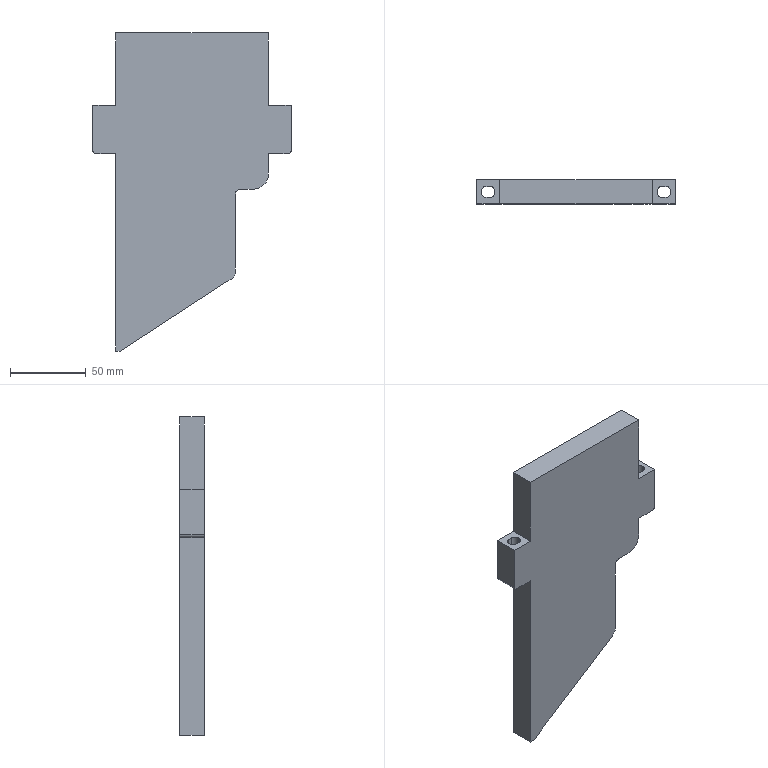Part | STEP file | 200 mesh_id2042 | 1 solid | 38 faces | box 131 x 16 x 210 mm | volume 283448 mm3 | plane 25 | cylinder 13 | commonest cylinder face diameters 6 x8 4 x2 6.5 x1 10 x1 20 x1
STEP:
#1=CARTESIAN_POINT('',(-16842.884,-3905.269,126.258));
#2=VERTEX_POINT('',#1);
#3=CARTESIAN_POINT('',(-16857.884,-3905.269,126.258));
#4=VERTEX_POINT('',#3);
#5=CARTESIAN_POINT('',(-16842.884,-3905.269,126.258));
#6=DIRECTION('',(-1.,0.,0.));
#7=VECTOR('',#6,1.);
#8=LINE('',#5,#7);
#9=EDGE_CURVE('',#2,#4,#8,.T.);
#10=ORIENTED_EDGE('',*,*,#9,.F.);
#11=CARTESIAN_POINT('',(-16842.884,-3889.269,126.258));
#12=VERTEX_POINT('',#11);
#13=CARTESIAN_POINT('',(-16842.884,-3889.269,126.258));
#14=DIRECTION('',(0.,-1.,0.));
#15=VECTOR('',#14,1.);
#16=LINE('',#13,#15);
#17=EDGE_CURVE('',#12,#2,#16,.T.);
#18=ORIENTED_EDGE('',*,*,#17,.F.);
#19=CARTESIAN_POINT('',(-16857.884,-3889.269,126.258));
#20=VERTEX_POINT('',#19);
#21=CARTESIAN_POINT('',(-16842.884,-3889.269,126.258));
#22=DIRECTION('',(-1.,0.,0.));
#23=VECTOR('',#22,1.);
#24=LINE('',#21,#23);
#25=EDGE_CURVE('',#12,#20,#24,.T.);
#26=ORIENTED_EDGE('',*,*,#25,.T.);
#27=CARTESIAN_POINT('',(-16857.884,-3889.269,126.258));
#28=DIRECTION('',(0.,-1.,0.));
#29=VECTOR('',#28,1.);
#30=LINE('',#27,#29);
#31=EDGE_CURVE('',#20,#4,#30,.T.);
#32=ORIENTED_EDGE('',*,*,#31,.T.);
#33=EDGE_LOOP('',(#10,#18,#26,#32));
#34=FACE_BOUND('',#33,.T.);
#35=CARTESIAN_POINT('',(-16851.884,-3893.769,126.258));
#36=VERTEX_POINT('',#35);
#37=CARTESIAN_POINT('',(-16848.884,-3893.769,126.258));
#38=VERTEX_POINT('',#37);
#39=CARTESIAN_POINT('',(-16842.884,-3893.769,126.258));
#40=DIRECTION('',(1.,0.,0.));
#41=VECTOR('',#40,1.);
#42=LINE('',#39,#41);
#43=EDGE_CURVE('',#36,#38,#42,.T.);
#44=ORIENTED_EDGE('',*,*,#43,.T.);
#45=CARTESIAN_POINT('',(-16845.884,-3896.769,126.258));
#46=VERTEX_POINT('',#45);
#47=CARTESIAN_POINT('',(-16848.884,-3896.769,126.258));
#48=DIRECTION('',(0.,0.,-1.));
#49=DIRECTION('',(-1.,0.,0.));
#50=AXIS2_PLACEMENT_3D('',#47,#48,#49);
#51=CIRCLE('',#50,3.);
#52=EDGE_CURVE('',#38,#46,#51,.T.);
#53=ORIENTED_EDGE('',*,*,#52,.T.);
#54=CARTESIAN_POINT('',(-16845.884,-3897.769,126.258));
#55=VERTEX_POINT('',#54);
#56=CARTESIAN_POINT('',(-16845.884,-3889.269,126.258));
#57=DIRECTION('',(0.,-1.,0.));
#58=VECTOR('',#57,1.);
#59=LINE('',#56,#58);
#60=EDGE_CURVE('',#46,#55,#59,.T.);
#61=ORIENTED_EDGE('',*,*,#60,.T.);
#62=CARTESIAN_POINT('',(-16848.884,-3900.769,126.258));
#63=VERTEX_POINT('',#62);
#64=CARTESIAN_POINT('',(-16848.884,-3897.769,126.258));
#65=DIRECTION('',(0.,0.,-1.));
#66=DIRECTION('',(-1.,0.,0.));
#67=AXIS2_PLACEMENT_3D('',#64,#65,#66);
#68=CIRCLE('',#67,3.);
#69=EDGE_CURVE('',#55,#63,#68,.T.);
#70=ORIENTED_EDGE('',*,*,#69,.T.);
#71=CARTESIAN_POINT('',(-16851.884,-3900.769,126.258));
#72=VERTEX_POINT('',#71);
#73=CARTESIAN_POINT('',(-16842.884,-3900.769,126.258));
#74=DIRECTION('',(-1.,0.,0.));
#75=VECTOR('',#74,1.);
#76=LINE('',#73,#75);
#77=EDGE_CURVE('',#63,#72,#76,.T.);
#78=ORIENTED_EDGE('',*,*,#77,.T.);
#79=CARTESIAN_POINT('',(-16854.884,-3897.769,126.258));
#80=VERTEX_POINT('',#79);
#81=CARTESIAN_POINT('',(-16851.884,-3897.769,126.258));
#82=DIRECTION('',(0.,0.,-1.));
#83=DIRECTION('',(-1.,0.,0.));
#84=AXIS2_PLACEMENT_3D('',#81,#82,#83);
#85=CIRCLE('',#84,3.);
#86=EDGE_CURVE('',#72,#80,#85,.T.);
#87=ORIENTED_EDGE('',*,*,#86,.T.);
#88=CARTESIAN_POINT('',(-16854.884,-3896.769,126.258));
#89=VERTEX_POINT('',#88);
#90=CARTESIAN_POINT('',(-16854.884,-3889.269,126.258));
#91=DIRECTION('',(0.,1.,0.));
#92=VECTOR('',#91,1.);
#93=LINE('',#90,#92);
#94=EDGE_CURVE('',#80,#89,#93,.T.);
#95=ORIENTED_EDGE('',*,*,#94,.T.);
#96=CARTESIAN_POINT('',(-16851.884,-3896.769,126.258));
#97=DIRECTION('',(0.,0.,-1.));
#98=DIRECTION('',(-1.,0.,0.));
#99=AXIS2_PLACEMENT_3D('',#96,#97,#98);
#100=CIRCLE('',#99,3.);
#101=EDGE_CURVE('',#89,#36,#100,.T.);
#102=ORIENTED_EDGE('',*,*,#101,.T.);
#103=EDGE_LOOP('',(#44,#53,#61,#70,#78,#87,#95,#102));
#104=FACE_BOUND('',#103,.T.);
#105=CARTESIAN_POINT('',(-16842.884,-3889.269,126.258));
#106=DIRECTION('',(0.,0.,-1.));
#107=DIRECTION('',(0.,-1.,0.));
#108=AXIS2_PLACEMENT_3D('',#105,#106,#107);
#109=PLANE('',#108);
#110=ADVANCED_FACE('',(#34,#104),#109,.F.);
#111=CARTESIAN_POINT('',(-16726.884,-3905.269,126.258));
#112=VERTEX_POINT('',#111);
#113=CARTESIAN_POINT('',(-16741.884,-3905.269,126.258));
#114=VERTEX_POINT('',#113);
#115=CARTESIAN_POINT('',(-16726.884,-3905.269,126.258));
#116=DIRECTION('',(-1.,0.,0.));
#117=VECTOR('',#116,1.);
#118=LINE('',#115,#117);
#119=EDGE_CURVE('',#112,#114,#118,.T.);
#120=ORIENTED_EDGE('',*,*,#119,.F.);
#121=CARTESIAN_POINT('',(-16726.884,-3889.269,126.258));
#122=VERTEX_POINT('',#121);
#123=CARTESIAN_POINT('',(-16726.884,-3889.269,126.258));
#124=DIRECTION('',(0.,-1.,0.));
#125=VECTOR('',#124,1.);
#126=LINE('',#123,#125);
#127=EDGE_CURVE('',#122,#112,#126,.T.);
#128=ORIENTED_EDGE('',*,*,#127,.F.);
#129=CARTESIAN_POINT('',(-16741.884,-3889.269,126.258));
#130=VERTEX_POINT('',#129);
#131=CARTESIAN_POINT('',(-16726.884,-3889.269,126.258));
#132=DIRECTION('',(-1.,0.,0.));
#133=VECTOR('',#132,1.);
#134=LINE('',#131,#133);
#135=EDGE_CURVE('',#122,#130,#134,.T.);
#136=ORIENTED_EDGE('',*,*,#135,.T.);
#137=CARTESIAN_POINT('',(-16741.884,-3889.269,126.258));
#138=DIRECTION('',(0.,-1.,0.));
#139=VECTOR('',#138,1.);
#140=LINE('',#137,#139);
#141=EDGE_CURVE('',#130,#114,#140,.T.);
#142=ORIENTED_EDGE('',*,*,#141,.T.);
#143=EDGE_LOOP('',(#120,#128,#136,#142));
#144=FACE_BOUND('',#143,.T.);
#145=CARTESIAN_POINT('',(-16738.884,-3897.769,126.258));
#146=VERTEX_POINT('',#145);
#147=CARTESIAN_POINT('',(-16738.884,-3896.769,126.258));
#148=VERTEX_POINT('',#147);
#149=CARTESIAN_POINT('',(-16738.884,-3889.269,126.258));
#150=DIRECTION('',(0.,1.,0.));
#151=VECTOR('',#150,1.);
#152=LINE('',#149,#151);
#153=EDGE_CURVE('',#146,#148,#152,.T.);
#154=ORIENTED_EDGE('',*,*,#153,.T.);
#155=CARTESIAN_POINT('',(-16735.884,-3893.769,126.258));
#156=VERTEX_POINT('',#155);
#157=CARTESIAN_POINT('',(-16735.884,-3896.769,126.258));
#158=DIRECTION('',(0.,0.,-1.));
#159=DIRECTION('',(-1.,0.,0.));
#160=AXIS2_PLACEMENT_3D('',#157,#158,#159);
#161=CIRCLE('',#160,3.);
#162=EDGE_CURVE('',#148,#156,#161,.T.);
#163=ORIENTED_EDGE('',*,*,#162,.T.);
#164=CARTESIAN_POINT('',(-16732.884,-3893.769,126.258));
#165=VERTEX_POINT('',#164);
#166=CARTESIAN_POINT('',(-16726.884,-3893.769,126.258));
#167=DIRECTION('',(1.,0.,0.));
#168=VECTOR('',#167,1.);
#169=LINE('',#166,#168);
#170=EDGE_CURVE('',#156,#165,#169,.T.);
#171=ORIENTED_EDGE('',*,*,#170,.T.);
#172=CARTESIAN_POINT('',(-16729.884,-3896.769,126.258));
#173=VERTEX_POINT('',#172);
#174=CARTESIAN_POINT('',(-16732.884,-3896.769,126.258));
#175=DIRECTION('',(0.,0.,-1.));
#176=DIRECTION('',(-1.,0.,0.));
#177=AXIS2_PLACEMENT_3D('',#174,#175,#176);
#178=CIRCLE('',#177,3.);
#179=EDGE_CURVE('',#165,#173,#178,.T.);
#180=ORIENTED_EDGE('',*,*,#179,.T.);
#181=CARTESIAN_POINT('',(-16729.884,-3897.769,126.258));
#182=VERTEX_POINT('',#181);
#183=CARTESIAN_POINT('',(-16729.884,-3889.269,126.258));
#184=DIRECTION('',(0.,-1.,0.));
#185=VECTOR('',#184,1.);
#186=LINE('',#183,#185);
#187=EDGE_CURVE('',#173,#182,#186,.T.);
#188=ORIENTED_EDGE('',*,*,#187,.T.);
#189=CARTESIAN_POINT('',(-16732.884,-3900.769,126.258));
#190=VERTEX_POINT('',#189);
#191=CARTESIAN_POINT('',(-16732.884,-3897.769,126.258));
#192=DIRECTION('',(0.,0.,-1.));
#193=DIRECTION('',(-1.,0.,0.));
#194=AXIS2_PLACEMENT_3D('',#191,#192,#193);
#195=CIRCLE('',#194,3.);
#196=EDGE_CURVE('',#182,#190,#195,.T.);
#197=ORIENTED_EDGE('',*,*,#196,.T.);
#198=CARTESIAN_POINT('',(-16735.884,-3900.769,126.258));
#199=VERTEX_POINT('',#198);
#200=CARTESIAN_POINT('',(-16726.884,-3900.769,126.258));
#201=DIRECTION('',(-1.,0.,0.));
#202=VECTOR('',#201,1.);
#203=LINE('',#200,#202);
#204=EDGE_CURVE('',#190,#199,#203,.T.);
#205=ORIENTED_EDGE('',*,*,#204,.T.);
#206=CARTESIAN_POINT('',(-16735.884,-3897.769,126.258));
#207=DIRECTION('',(0.,0.,-1.));
#208=DIRECTION('',(-1.,0.,0.));
#209=AXIS2_PLACEMENT_3D('',#206,#207,#208);
#210=CIRCLE('',#209,3.);
#211=EDGE_CURVE('',#199,#146,#210,.T.);
#212=ORIENTED_EDGE('',*,*,#211,.T.);
#213=EDGE_LOOP('',(#154,#163,#171,#180,#188,#197,#205,#212));
#214=FACE_BOUND('',#213,.T.);
#215=CARTESIAN_POINT('',(-16726.884,-3889.269,126.258));
#216=DIRECTION('',(0.,0.,-1.));
#217=DIRECTION('',(0.,-1.,0.));
#218=AXIS2_PLACEMENT_3D('',#215,#216,#217);
#219=PLANE('',#218);
#220=ADVANCED_FACE('',(#144,#214),#219,.F.);
#221=CARTESIAN_POINT('',(-16763.684,-3905.269,67.499));
#222=VERTEX_POINT('',#221);
#223=CARTESIAN_POINT('',(-16760.434,-3905.269,70.749));
#224=VERTEX_POINT('',#223);
#225=CARTESIAN_POINT('',(-16760.434,-3905.269,67.499));
#226=DIRECTION('',(0.,1.,0.));
#227=DIRECTION('',(0.,0.,-1.));
#228=AXIS2_PLACEMENT_3D('',#225,#226,#227);
#229=CIRCLE('',#228,3.25);
#230=EDGE_CURVE('',#222,#224,#229,.T.);
#231=ORIENTED_EDGE('',*,*,#230,.F.);
#232=CARTESIAN_POINT('',(-16763.684,-3889.269,67.499));
#233=VERTEX_POINT('',#232);
#234=CARTESIAN_POINT('',(-16763.684,-3889.269,67.499));
#235=DIRECTION('',(0.,-1.,0.));
#236=VECTOR('',#235,1.);
#237=LINE('',#234,#236);
#238=EDGE_CURVE('',#233,#222,#237,.T.);
#239=ORIENTED_EDGE('',*,*,#238,.F.);
#240=CARTESIAN_POINT('',(-16760.434,-3889.269,70.749));
#241=VERTEX_POINT('',#240);
#242=CARTESIAN_POINT('',(-16760.434,-3889.269,67.499));
#243=DIRECTION('',(0.,1.,0.));
#244=DIRECTION('',(0.,0.,-1.));
#245=AXIS2_PLACEMENT_3D('',#242,#243,#244);
#246=CIRCLE('',#245,3.25);
#247=EDGE_CURVE('',#233,#241,#246,.T.);
#248=ORIENTED_EDGE('',*,*,#247,.T.);
#249=CARTESIAN_POINT('',(-16760.434,-3889.269,70.749));
#250=DIRECTION('',(0.,-1.,0.));
#251=VECTOR('',#250,1.);
#252=LINE('',#249,#251);
#253=EDGE_CURVE('',#241,#224,#252,.T.);
#254=ORIENTED_EDGE('',*,*,#253,.T.);
#255=EDGE_LOOP('',(#231,#239,#248,#254));
#256=FACE_OUTER_BOUND('',#255,.T.);
#257=CARTESIAN_POINT('',(-16760.434,-3889.269,67.499));
#258=DIRECTION('',(0.,-1.,0.));
#259=DIRECTION('',(-1.,0.,0.));
#260=AXIS2_PLACEMENT_3D('',#257,#258,#259);
#261=CYLINDRICAL_SURFACE('',#260,3.25);
#262=ADVANCED_FACE('',(#256),#261,.F.);
#263=CARTESIAN_POINT('',(-16751.884,-3889.269,70.749));
#264=VERTEX_POINT('',#263);
#265=CARTESIAN_POINT('',(-16760.434,-3889.269,70.749));
#266=DIRECTION('',(1.,0.,0.));
#267=VECTOR('',#266,1.);
#268=LINE('',#265,#267);
#269=EDGE_CURVE('',#241,#264,#268,.T.);
#270=ORIENTED_EDGE('',*,*,#269,.T.);
#271=CARTESIAN_POINT('',(-16751.884,-3905.269,70.749));
#272=VERTEX_POINT('',#271);
#273=CARTESIAN_POINT('',(-16751.884,-3889.269,70.749));
#274=DIRECTION('',(0.,-1.,0.));
#275=VECTOR('',#274,1.);
#276=LINE('',#273,#275);
#277=EDGE_CURVE('',#264,#272,#276,.T.);
#278=ORIENTED_EDGE('',*,*,#277,.T.);
#279=CARTESIAN_POINT('',(-16760.434,-3905.269,70.749));
#280=DIRECTION('',(1.,0.,0.));
#281=VECTOR('',#280,1.);
#282=LINE('',#279,#281);
#283=EDGE_CURVE('',#224,#272,#282,.T.);
#284=ORIENTED_EDGE('',*,*,#283,.F.);
#285=ORIENTED_EDGE('',*,*,#253,.F.);
#286=EDGE_LOOP('',(#270,#278,#284,#285));
#287=FACE_OUTER_BOUND('',#286,.T.);
#288=CARTESIAN_POINT('',(-16760.434,-3889.269,70.749));
#289=DIRECTION('',(0.,0.,1.));
#290=DIRECTION('',(-1.,0.,0.));
#291=AXIS2_PLACEMENT_3D('',#288,#289,#290);
#292=PLANE('',#291);
#293=ADVANCED_FACE('',(#287),#292,.F.);
#294=CARTESIAN_POINT('',(-16741.884,-3905.269,80.749));
#295=VERTEX_POINT('',#294);
#296=CARTESIAN_POINT('',(-16741.884,-3905.269,94.258));
#297=VERTEX_POINT('',#296);
#298=CARTESIAN_POINT('',(-16741.884,-3905.269,72.499));
#299=DIRECTION('',(0.,0.,1.));
#300=VECTOR('',#299,1.);
#301=LINE('',#298,#300);
#302=EDGE_CURVE('',#295,#297,#301,.T.);
#303=ORIENTED_EDGE('',*,*,#302,.F.);
#304=CARTESIAN_POINT('',(-16741.884,-3889.269,80.749));
#305=VERTEX_POINT('',#304);
#306=CARTESIAN_POINT('',(-16741.884,-3889.269,80.749));
#307=DIRECTION('',(0.,1.,0.));
#308=VECTOR('',#307,1.);
#309=LINE('',#306,#308);
#310=EDGE_CURVE('',#295,#305,#309,.T.);
#311=ORIENTED_EDGE('',*,*,#310,.T.);
#312=CARTESIAN_POINT('',(-16741.884,-3889.269,94.258));
#313=VERTEX_POINT('',#312);
#314=CARTESIAN_POINT('',(-16741.884,-3889.269,72.499));
#315=DIRECTION('',(0.,0.,1.));
#316=VECTOR('',#315,1.);
#317=LINE('',#314,#316);
#318=EDGE_CURVE('',#305,#313,#317,.T.);
#319=ORIENTED_EDGE('',*,*,#318,.T.);
#320=CARTESIAN_POINT('',(-16741.884,-3889.269,94.258));
#321=DIRECTION('',(0.,-1.,0.));
#322=VECTOR('',#321,1.);
#323=LINE('',#320,#322);
#324=EDGE_CURVE('',#313,#297,#323,.T.);
#325=ORIENTED_EDGE('',*,*,#324,.T.);
#326=EDGE_LOOP('',(#303,#311,#319,#325));
#327=FACE_OUTER_BOUND('',#326,.T.);
#328=CARTESIAN_POINT('',(-16741.884,-3889.269,72.499));
#329=DIRECTION('',(-1.,0.,0.));
#330=DIRECTION('',(0.,1.,0.));
#331=AXIS2_PLACEMENT_3D('',#328,#329,#330);
#332=PLANE('',#331);
#333=ADVANCED_FACE('',(#327),#332,.F.);
#334=CARTESIAN_POINT('',(-16735.884,-3900.769,94.258));
#335=VERTEX_POINT('',#334);
#336=CARTESIAN_POINT('',(-16738.884,-3897.769,94.258));
#337=VERTEX_POINT('',#336);
#338=CARTESIAN_POINT('',(-16735.884,-3897.769,94.258));
#339=DIRECTION('',(0.,0.,-1.));
#340=DIRECTION('',(1.,0.,0.));
#341=AXIS2_PLACEMENT_3D('',#338,#339,#340);
#342=CIRCLE('',#341,3.);
#343=EDGE_CURVE('',#335,#337,#342,.T.);
#344=ORIENTED_EDGE('',*,*,#343,.F.);
#345=CARTESIAN_POINT('',(-16732.884,-3900.769,94.258));
#346=VERTEX_POINT('',#345);
#347=CARTESIAN_POINT('',(-16741.884,-3900.769,94.258));
#348=DIRECTION('',(-1.,0.,0.));
#349=VECTOR('',#348,1.);
#350=LINE('',#347,#349);
#351=EDGE_CURVE('',#346,#335,#350,.T.);
#352=ORIENTED_EDGE('',*,*,#351,.F.);
#353=CARTESIAN_POINT('',(-16729.884,-3897.769,94.258));
#354=VERTEX_POINT('',#353);
#355=CARTESIAN_POINT('',(-16732.884,-3897.769,94.258));
#356=DIRECTION('',(0.,0.,-1.));
#357=DIRECTION('',(1.,0.,0.));
#358=AXIS2_PLACEMENT_3D('',#355,#356,#357);
#359=CIRCLE('',#358,3.);
#360=EDGE_CURVE('',#354,#346,#359,.T.);
#361=ORIENTED_EDGE('',*,*,#360,.F.);
#362=CARTESIAN_POINT('',(-16729.884,-3896.769,94.258));
#363=VERTEX_POINT('',#362);
#364=CARTESIAN_POINT('',(-16729.884,-3889.269,94.258));
#365=DIRECTION('',(0.,-1.,0.));
#366=VECTOR('',#365,1.);
#367=LINE('',#364,#366);
#368=EDGE_CURVE('',#363,#354,#367,.T.);
#369=ORIENTED_EDGE('',*,*,#368,.F.);
#370=CARTESIAN_POINT('',(-16732.884,-3893.769,94.258));
#371=VERTEX_POINT('',#370);
#372=CARTESIAN_POINT('',(-16732.884,-3896.769,94.258));
#373=DIRECTION('',(0.,0.,-1.));
#374=DIRECTION('',(1.,0.,0.));
#375=AXIS2_PLACEMENT_3D('',#372,#373,#374);
#376=CIRCLE('',#375,3.);
#377=EDGE_CURVE('',#371,#363,#376,.T.);
#378=ORIENTED_EDGE('',*,*,#377,.F.);
#379=CARTESIAN_POINT('',(-16735.884,-3893.769,94.258));
#380=VERTEX_POINT('',#379);
#381=CARTESIAN_POINT('',(-16741.884,-3893.769,94.258));
#382=DIRECTION('',(1.,0.,0.));
#383=VECTOR('',#382,1.);
#384=LINE('',#381,#383);
#385=EDGE_CURVE('',#380,#371,#384,.T.);
#386=ORIENTED_EDGE('',*,*,#385,.F.);
#387=CARTESIAN_POINT('',(-16738.884,-3896.769,94.258));
#388=VERTEX_POINT('',#387);
#389=CARTESIAN_POINT('',(-16735.884,-3896.769,94.258));
#390=DIRECTION('',(0.,0.,-1.));
#391=DIRECTION('',(1.,0.,0.));
#392=AXIS2_PLACEMENT_3D('',#389,#390,#391);
#393=CIRCLE('',#392,3.);
#394=EDGE_CURVE('',#388,#380,#393,.T.);
#395=ORIENTED_EDGE('',*,*,#394,.F.);
#396=CARTESIAN_POINT('',(-16738.884,-3889.269,94.258));
#397=DIRECTION('',(0.,1.,0.));
#398=VECTOR('',#397,1.);
#399=LINE('',#396,#398);
#400=EDGE_CURVE('',#337,#388,#399,.T.);
#401=ORIENTED_EDGE('',*,*,#400,.F.);
#402=EDGE_LOOP('',(#344,#352,#361,#369,#378,#386,#395,#401));
#403=FACE_BOUND('',#402,.T.);
#404=CARTESIAN_POINT('',(-16728.884,-3889.269,94.258));
#405=VERTEX_POINT('',#404);
#406=CARTESIAN_POINT('',(-16741.884,-3889.269,94.258));
#407=DIRECTION('',(1.,0.,0.));
#408=VECTOR('',#407,1.);
#409=LINE('',#406,#408);
#410=EDGE_CURVE('',#313,#405,#409,.T.);
#411=ORIENTED_EDGE('',*,*,#410,.T.);
#412=CARTESIAN_POINT('',(-16728.884,-3905.269,94.258));
#413=VERTEX_POINT('',#412);
#414=CARTESIAN_POINT('',(-16728.884,-3889.269,94.258));
#415=DIRECTION('',(0.,-1.,0.));
#416=VECTOR('',#415,1.);
#417=LINE('',#414,#416);
#418=EDGE_CURVE('',#405,#413,#417,.T.);
#419=ORIENTED_EDGE('',*,*,#418,.T.);
#420=CARTESIAN_POINT('',(-16741.884,-3905.269,94.258));
#421=DIRECTION('',(1.,0.,0.));
#422=VECTOR('',#421,1.);
#423=LINE('',#420,#422);
#424=EDGE_CURVE('',#297,#413,#423,.T.);
#425=ORIENTED_EDGE('',*,*,#424,.F.);
#426=ORIENTED_EDGE('',*,*,#324,.F.);
#427=EDGE_LOOP('',(#411,#419,#425,#426));
#428=FACE_BOUND('',#427,.T.);
#429=CARTESIAN_POINT('',(-16741.884,-3889.269,94.258));
#430=DIRECTION('',(0.,0.,1.));
#431=DIRECTION('',(0.,1.,0.));
#432=AXIS2_PLACEMENT_3D('',#429,#430,#431);
#433=PLANE('',#432);
#434=ADVANCED_FACE('',(#403,#428),#433,.F.);
#435=CARTESIAN_POINT('',(-16726.884,-3905.269,96.258));
#436=VERTEX_POINT('',#435);
#437=CARTESIAN_POINT('',(-16726.884,-3905.269,94.258));
#438=DIRECTION('',(0.,0.,1.));
#439=VECTOR('',#438,1.);
#440=LINE('',#437,#439);
#441=EDGE_CURVE('',#436,#112,#440,.T.);
#442=ORIENTED_EDGE('',*,*,#441,.F.);
#443=CARTESIAN_POINT('',(-16726.884,-3889.269,96.258));
#444=VERTEX_POINT('',#443);
#445=CARTESIAN_POINT('',(-16726.884,-3889.269,96.258));
#446=DIRECTION('',(0.,1.,0.));
#447=VECTOR('',#446,1.);
#448=LINE('',#445,#447);
#449=EDGE_CURVE('',#436,#444,#448,.T.);
#450=ORIENTED_EDGE('',*,*,#449,.T.);
#451=CARTESIAN_POINT('',(-16726.884,-3889.269,94.258));
#452=DIRECTION('',(0.,0.,1.));
#453=VECTOR('',#452,1.);
#454=LINE('',#451,#453);
#455=EDGE_CURVE('',#444,#122,#454,.T.);
#456=ORIENTED_EDGE('',*,*,#455,.T.);
#457=ORIENTED_EDGE('',*,*,#127,.T.);
#458=EDGE_LOOP('',(#442,#450,#456,#457));
#459=FACE_OUTER_BOUND('',#458,.T.);
#460=CARTESIAN_POINT('',(-16726.884,-3889.269,94.258));
#461=DIRECTION('',(-1.,0.,0.));
#462=DIRECTION('',(0.,1.,0.));
#463=AXIS2_PLACEMENT_3D('',#460,#461,#462);
#464=PLANE('',#463);
#465=ADVANCED_FACE('',(#459),#464,.F.);
#466=CARTESIAN_POINT('',(-16741.884,-3905.269,173.87));
#467=VERTEX_POINT('',#466);
#468=CARTESIAN_POINT('',(-16741.884,-3905.269,124.258));
#469=DIRECTION('',(0.,0.,1.));
#470=VECTOR('',#469,1.);
#471=LINE('',#468,#470);
#472=EDGE_CURVE('',#114,#467,#471,.T.);
#473=ORIENTED_EDGE('',*,*,#472,.F.);
#474=ORIENTED_EDGE('',*,*,#141,.F.);
#475=CARTESIAN_POINT('',(-16741.884,-3889.269,173.87));
#476=VERTEX_POINT('',#475);
#477=CARTESIAN_POINT('',(-16741.884,-3889.269,124.258));
#478=DIRECTION('',(0.,0.,1.));
#479=VECTOR('',#478,1.);
#480=LINE('',#477,#479);
#481=EDGE_CURVE('',#130,#476,#480,.T.);
#482=ORIENTED_EDGE('',*,*,#481,.T.);
#483=CARTESIAN_POINT('',(-16741.884,-3889.269,173.87));
#484=DIRECTION('',(0.,-1.,0.));
#485=VECTOR('',#484,1.);
#486=LINE('',#483,#485);
#487=EDGE_CURVE('',#476,#467,#486,.T.);
#488=ORIENTED_EDGE('',*,*,#487,.T.);
#489=EDGE_LOOP('',(#473,#474,#482,#488));
#490=FACE_OUTER_BOUND('',#489,.T.);
#491=CARTESIAN_POINT('',(-16741.884,-3889.269,124.258));
#492=DIRECTION('',(-1.,0.,0.));
#493=DIRECTION('',(0.,1.,0.));
#494=AXIS2_PLACEMENT_3D('',#491,#492,#493);
#495=PLANE('',#494);
#496=ADVANCED_FACE('',(#490),#495,.F.);
#497=CARTESIAN_POINT('',(-16842.884,-3905.269,173.87));
#498=VERTEX_POINT('',#497);
#499=CARTESIAN_POINT('',(-16731.884,-3905.269,173.87));
#500=DIRECTION('',(-1.,0.,0.));
#501=VECTOR('',#500,1.);
#502=LINE('',#499,#501);
#503=EDGE_CURVE('',#467,#498,#502,.T.);
#504=ORIENTED_EDGE('',*,*,#503,.F.);
#505=ORIENTED_EDGE('',*,*,#487,.F.);
#506=CARTESIAN_POINT('',(-16842.884,-3889.269,173.87));
#507=VERTEX_POINT('',#506);
#508=CARTESIAN_POINT('',(-16731.884,-3889.269,173.87));
#509=DIRECTION('',(-1.,0.,0.));
#510=VECTOR('',#509,1.);
#511=LINE('',#508,#510);
#512=EDGE_CURVE('',#476,#507,#511,.T.);
#513=ORIENTED_EDGE('',*,*,#512,.T.);
#514=CARTESIAN_POINT('',(-16842.884,-3889.269,173.87));
#515=DIRECTION('',(0.,-1.,0.));
#516=VECTOR('',#515,1.);
#517=LINE('',#514,#516);
#518=EDGE_CURVE('',#507,#498,#517,.T.);
#519=ORIENTED_EDGE('',*,*,#518,.T.);
#520=EDGE_LOOP('',(#504,#505,#513,#519));
#521=FACE_OUTER_BOUND('',#520,.T.);
#522=CARTESIAN_POINT('',(-16731.884,-3889.269,173.87));
#523=DIRECTION('',(0.,0.,-1.));
#524=DIRECTION('',(0.,-1.,0.));
#525=AXIS2_PLACEMENT_3D('',#522,#523,#524);
#526=PLANE('',#525);
#527=ADVANCED_FACE('',(#521),#526,.F.);
#528=CARTESIAN_POINT('',(-16842.884,-3905.269,153.87));
#529=DIRECTION('',(0.,0.,-1.));
#530=VECTOR('',#529,1.);
#531=LINE('',#528,#530);
#532=EDGE_CURVE('',#498,#2,#531,.T.);
#533=ORIENTED_EDGE('',*,*,#532,.F.);
#534=ORIENTED_EDGE('',*,*,#518,.F.);
#535=CARTESIAN_POINT('',(-16842.884,-3889.269,153.87));
#536=DIRECTION('',(0.,0.,-1.));
#537=VECTOR('',#536,1.);
#538=LINE('',#535,#537);
#539=EDGE_CURVE('',#507,#12,#538,.T.);
#540=ORIENTED_EDGE('',*,*,#539,.T.);
#541=ORIENTED_EDGE('',*,*,#17,.T.);
#542=EDGE_LOOP('',(#533,#534,#540,#541));
#543=FACE_OUTER_BOUND('',#542,.T.);
#544=CARTESIAN_POINT('',(-16842.884,-3889.269,153.87));
#545=DIRECTION('',(1.,0.,0.));
#546=DIRECTION('',(0.,-1.,0.));
#547=AXIS2_PLACEMENT_3D('',#544,#545,#546);
#548=PLANE('',#547);
#549=ADVANCED_FACE('',(#543),#548,.F.);
#550=CARTESIAN_POINT('',(-16857.884,-3889.269,96.258));
#551=VERTEX_POINT('',#550);
#552=CARTESIAN_POINT('',(-16857.884,-3889.269,124.258));
#553=DIRECTION('',(0.,0.,-1.));
#554=VECTOR('',#553,1.);
#555=LINE('',#552,#554);
#556=EDGE_CURVE('',#20,#551,#555,.T.);
#557=ORIENTED_EDGE('',*,*,#556,.T.);
#558=CARTESIAN_POINT('',(-16857.884,-3905.269,96.258));
#559=VERTEX_POINT('',#558);
#560=CARTESIAN_POINT('',(-16857.884,-3889.269,96.258));
#561=DIRECTION('',(0.,-1.,0.));
#562=VECTOR('',#561,1.);
#563=LINE('',#560,#562);
#564=EDGE_CURVE('',#551,#559,#563,.T.);
#565=ORIENTED_EDGE('',*,*,#564,.T.);
#566=CARTESIAN_POINT('',(-16857.884,-3905.269,124.258));
#567=DIRECTION('',(0.,0.,-1.));
#568=VECTOR('',#567,1.);
#569=LINE('',#566,#568);
#570=EDGE_CURVE('',#4,#559,#569,.T.);
#571=ORIENTED_EDGE('',*,*,#570,.F.);
#572=ORIENTED_EDGE('',*,*,#31,.F.);
#573=EDGE_LOOP('',(#557,#565,#571,#572));
#574=FACE_OUTER_BOUND('',#573,.T.);
#575=CARTESIAN_POINT('',(-16857.884,-3889.269,124.258));
#576=DIRECTION('',(1.,0.,0.));
#577=DIRECTION('',(0.,-1.,0.));
#578=AXIS2_PLACEMENT_3D('',#575,#576,#577);
#579=PLANE('',#578);
#580=ADVANCED_FACE('',(#574),#579,.F.);
#581=CARTESIAN_POINT('',(-16854.884,-3896.769,94.258));
#582=VERTEX_POINT('',#581);
#583=CARTESIAN_POINT('',(-16851.884,-3893.769,94.258));
#584=VERTEX_POINT('',#583);
#585=CARTESIAN_POINT('',(-16851.884,-3896.769,94.258));
#586=DIRECTION('',(0.,0.,-1.));
#587=DIRECTION('',(1.,0.,0.));
#588=AXIS2_PLACEMENT_3D('',#585,#586,#587);
#589=CIRCLE('',#588,3.);
#590=EDGE_CURVE('',#582,#584,#589,.T.);
#591=ORIENTED_EDGE('',*,*,#590,.F.);
#592=CARTESIAN_POINT('',(-16854.884,-3897.769,94.258));
#593=VERTEX_POINT('',#592);
#594=CARTESIAN_POINT('',(-16854.884,-3889.269,94.258));
#595=DIRECTION('',(0.,1.,0.));
#596=VECTOR('',#595,1.);
#597=LINE('',#594,#596);
#598=EDGE_CURVE('',#593,#582,#597,.T.);
#599=ORIENTED_EDGE('',*,*,#598,.F.);
#600=CARTESIAN_POINT('',(-16851.884,-3900.769,94.258));
#601=VERTEX_POINT('',#600);
#602=CARTESIAN_POINT('',(-16851.884,-3897.769,94.258));
#603=DIRECTION('',(0.,0.,-1.));
#604=DIRECTION('',(1.,0.,0.));
#605=AXIS2_PLACEMENT_3D('',#602,#603,#604);
#606=CIRCLE('',#605,3.);
#607=EDGE_CURVE('',#601,#593,#606,.T.);
#608=ORIENTED_EDGE('',*,*,#607,.F.);
#609=CARTESIAN_POINT('',(-16848.884,-3900.769,94.258));
#610=VERTEX_POINT('',#609);
#611=CARTESIAN_POINT('',(-16857.884,-3900.769,94.258));
#612=DIRECTION('',(-1.,0.,0.));
#613=VECTOR('',#612,1.);
#614=LINE('',#611,#613);
#615=EDGE_CURVE('',#610,#601,#614,.T.);
#616=ORIENTED_EDGE('',*,*,#615,.F.);
#617=CARTESIAN_POINT('',(-16845.884,-3897.769,94.258));
#618=VERTEX_POINT('',#617);
#619=CARTESIAN_POINT('',(-16848.884,-3897.769,94.258));
#620=DIRECTION('',(0.,0.,-1.));
#621=DIRECTION('',(1.,0.,0.));
#622=AXIS2_PLACEMENT_3D('',#619,#620,#621);
#623=CIRCLE('',#622,3.);
#624=EDGE_CURVE('',#618,#610,#623,.T.);
#625=ORIENTED_EDGE('',*,*,#624,.F.);
#626=CARTESIAN_POINT('',(-16845.884,-3896.769,94.258));
#627=VERTEX_POINT('',#626);
#628=CARTESIAN_POINT('',(-16845.884,-3889.269,94.258));
#629=DIRECTION('',(0.,-1.,0.));
#630=VECTOR('',#629,1.);
#631=LINE('',#628,#630);
#632=EDGE_CURVE('',#627,#618,#631,.T.);
#633=ORIENTED_EDGE('',*,*,#632,.F.);
#634=CARTESIAN_POINT('',(-16848.884,-3893.769,94.258));
#635=VERTEX_POINT('',#634);
#636=CARTESIAN_POINT('',(-16848.884,-3896.769,94.258));
#637=DIRECTION('',(0.,0.,-1.));
#638=DIRECTION('',(1.,0.,0.));
#639=AXIS2_PLACEMENT_3D('',#636,#637,#638);
#640=CIRCLE('',#639,3.);
#641=EDGE_CURVE('',#635,#627,#640,.T.);
#642=ORIENTED_EDGE('',*,*,#641,.F.);
#643=CARTESIAN_POINT('',(-16857.884,-3893.769,94.258));
#644=DIRECTION('',(1.,0.,0.));
#645=VECTOR('',#644,1.);
#646=LINE('',#643,#645);
#647=EDGE_CURVE('',#584,#635,#646,.T.);
#648=ORIENTED_EDGE('',*,*,#647,.F.);
#649=EDGE_LOOP('',(#591,#599,#608,#616,#625,#633,#642,#648));
#650=FACE_BOUND('',#649,.T.);
#651=CARTESIAN_POINT('',(-16855.884,-3905.269,94.258));
#652=VERTEX_POINT('',#651);
#653=CARTESIAN_POINT('',(-16842.884,-3905.269,94.258));
#654=VERTEX_POINT('',#653);
#655=CARTESIAN_POINT('',(-16857.884,-3905.269,94.258));
#656=DIRECTION('',(1.,0.,0.));
#657=VECTOR('',#656,1.);
#658=LINE('',#655,#657);
#659=EDGE_CURVE('',#652,#654,#658,.T.);
#660=ORIENTED_EDGE('',*,*,#659,.F.);
#661=CARTESIAN_POINT('',(-16855.884,-3889.269,94.258));
#662=VERTEX_POINT('',#661);
#663=CARTESIAN_POINT('',(-16855.884,-3889.269,94.258));
#664=DIRECTION('',(0.,1.,0.));
#665=VECTOR('',#664,1.);
#666=LINE('',#663,#665);
#667=EDGE_CURVE('',#652,#662,#666,.T.);
#668=ORIENTED_EDGE('',*,*,#667,.T.);
#669=CARTESIAN_POINT('',(-16842.884,-3889.269,94.258));
#670=VERTEX_POINT('',#669);
#671=CARTESIAN_POINT('',(-16857.884,-3889.269,94.258));
#672=DIRECTION('',(1.,0.,0.));
#673=VECTOR('',#672,1.);
#674=LINE('',#671,#673);
#675=EDGE_CURVE('',#662,#670,#674,.T.);
#676=ORIENTED_EDGE('',*,*,#675,.T.);
#677=CARTESIAN_POINT('',(-16842.884,-3889.269,94.258));
#678=DIRECTION('',(0.,-1.,0.));
#679=VECTOR('',#678,1.);
#680=LINE('',#677,#679);
#681=EDGE_CURVE('',#670,#654,#680,.T.);
#682=ORIENTED_EDGE('',*,*,#681,.T.);
#683=EDGE_LOOP('',(#660,#668,#676,#682));
#684=FACE_BOUND('',#683,.T.);
#685=CARTESIAN_POINT('',(-16857.884,-3889.269,94.258));
#686=DIRECTION('',(0.,0.,1.));
#687=DIRECTION('',(0.,1.,0.));
#688=AXIS2_PLACEMENT_3D('',#685,#686,#687);
#689=PLANE('',#688);
#690=ADVANCED_FACE('',(#650,#684),#689,.F.);
#691=CARTESIAN_POINT('',(-16842.884,-3905.269,-36.13));
#692=VERTEX_POINT('',#691);
#693=CARTESIAN_POINT('',(-16842.884,-3905.269,94.258));
#694=DIRECTION('',(0.,0.,-1.));
#695=VECTOR('',#694,1.);
#696=LINE('',#693,#695);
#697=EDGE_CURVE('',#654,#692,#696,.T.);
#698=ORIENTED_EDGE('',*,*,#697,.F.);
#699=ORIENTED_EDGE('',*,*,#681,.F.);
#700=CARTESIAN_POINT('',(-16842.884,-3889.269,-36.13));
#701=VERTEX_POINT('',#700);
#702=CARTESIAN_POINT('',(-16842.884,-3889.269,94.258));
#703=DIRECTION('',(0.,0.,-1.));
#704=VECTOR('',#703,1.);
#705=LINE('',#702,#704);
#706=EDGE_CURVE('',#670,#701,#705,.T.);
#707=ORIENTED_EDGE('',*,*,#706,.T.);
#708=CARTESIAN_POINT('',(-16842.884,-3889.269,-36.13));
#709=DIRECTION('',(0.,-1.,0.));
#710=VECTOR('',#709,1.);
#711=LINE('',#708,#710);
#712=EDGE_CURVE('',#701,#692,#711,.T.);
#713=ORIENTED_EDGE('',*,*,#712,.T.);
#714=EDGE_LOOP('',(#698,#699,#707,#713));
#715=FACE_OUTER_BOUND('',#714,.T.);
#716=CARTESIAN_POINT('',(-16842.884,-3889.269,94.258));
#717=DIRECTION('',(1.,0.,0.));
#718=DIRECTION('',(0.,-1.,0.));
#719=AXIS2_PLACEMENT_3D('',#716,#717,#718);
#720=PLANE('',#719);
#721=ADVANCED_FACE('',(#715),#720,.F.);
#722=CARTESIAN_POINT('',(-16839.804,-3905.269,-36.13));
#723=VERTEX_POINT('',#722);
#724=CARTESIAN_POINT('',(-16842.884,-3905.269,-36.13));
#725=DIRECTION('',(1.,0.,0.));
#726=VECTOR('',#725,1.);
#727=LINE('',#724,#726);
#728=EDGE_CURVE('',#692,#723,#727,.T.);
#729=ORIENTED_EDGE('',*,*,#728,.F.);
#730=ORIENTED_EDGE('',*,*,#712,.F.);
#731=CARTESIAN_POINT('',(-16839.804,-3889.269,-36.13));
#732=VERTEX_POINT('',#731);
#733=CARTESIAN_POINT('',(-16842.884,-3889.269,-36.13));
#734=DIRECTION('',(1.,0.,0.));
#735=VECTOR('',#734,1.);
#736=LINE('',#733,#735);
#737=EDGE_CURVE('',#701,#732,#736,.T.);
#738=ORIENTED_EDGE('',*,*,#737,.T.);
#739=CARTESIAN_POINT('',(-16839.804,-3889.269,-36.13));
#740=DIRECTION('',(0.,-1.,0.));
#741=VECTOR('',#740,1.);
#742=LINE('',#739,#741);
#743=EDGE_CURVE('',#732,#723,#742,.T.);
#744=ORIENTED_EDGE('',*,*,#743,.T.);
#745=EDGE_LOOP('',(#729,#730,#738,#744));
#746=FACE_OUTER_BOUND('',#745,.T.);
#747=CARTESIAN_POINT('',(-16842.884,-3889.269,-36.13));
#748=DIRECTION('',(0.,0.,1.));
#749=DIRECTION('',(0.,1.,0.));
#750=AXIS2_PLACEMENT_3D('',#747,#748,#749);
#751=PLANE('',#750);
#752=ADVANCED_FACE('',(#746),#751,.F.);
#753=CARTESIAN_POINT('',(-16765.961,-3889.269,11.825));
#754=VERTEX_POINT('',#753);
#755=CARTESIAN_POINT('',(-16839.804,-3889.269,-36.13));
#756=DIRECTION('',(0.8387,0.,0.5446));
#757=VECTOR('',#756,1.);
#758=LINE('',#755,#757);
#759=EDGE_CURVE('',#732,#754,#758,.T.);
#760=ORIENTED_EDGE('',*,*,#759,.T.);
#761=CARTESIAN_POINT('',(-16765.961,-3905.269,11.825));
#762=VERTEX_POINT('',#761);
#763=CARTESIAN_POINT('',(-16765.961,-3889.269,11.825));
#764=DIRECTION('',(0.,-1.,0.));
#765=VECTOR('',#764,1.);
#766=LINE('',#763,#765);
#767=EDGE_CURVE('',#754,#762,#766,.T.);
#768=ORIENTED_EDGE('',*,*,#767,.T.);
#769=CARTESIAN_POINT('',(-16839.804,-3905.269,-36.13));
#770=DIRECTION('',(0.8387,0.,0.5446));
#771=VECTOR('',#770,1.);
#772=LINE('',#769,#771);
#773=EDGE_CURVE('',#723,#762,#772,.T.);
#774=ORIENTED_EDGE('',*,*,#773,.F.);
#775=ORIENTED_EDGE('',*,*,#743,.F.);
#776=EDGE_LOOP('',(#760,#768,#774,#775));
#777=FACE_OUTER_BOUND('',#776,.T.);
#778=CARTESIAN_POINT('',(-16839.804,-3889.269,-36.13));
#779=DIRECTION('',(-0.5446,0.,0.8387));
#780=DIRECTION('',(-0.8387,0.,-0.5446));
#781=AXIS2_PLACEMENT_3D('',#778,#779,#780);
#782=PLANE('',#781);
#783=ADVANCED_FACE('',(#777),#782,.F.);
#784=CARTESIAN_POINT('',(-16763.684,-3905.269,16.018));
#785=VERTEX_POINT('',#784);
#786=CARTESIAN_POINT('',(-16763.684,-3905.269,53.944));
#787=DIRECTION('',(0.,0.,1.));
#788=VECTOR('',#787,1.);
#789=LINE('',#786,#788);
#790=EDGE_CURVE('',#785,#222,#789,.T.);
#791=ORIENTED_EDGE('',*,*,#790,.F.);
#792=CARTESIAN_POINT('',(-16763.684,-3889.269,16.018));
#793=VERTEX_POINT('',#792);
#794=CARTESIAN_POINT('',(-16763.684,-3889.269,16.018));
#795=DIRECTION('',(0.,1.,0.));
#796=VECTOR('',#795,1.);
#797=LINE('',#794,#796);
#798=EDGE_CURVE('',#785,#793,#797,.T.);
#799=ORIENTED_EDGE('',*,*,#798,.T.);
#800=CARTESIAN_POINT('',(-16763.684,-3889.269,53.944));
#801=DIRECTION('',(0.,0.,1.));
#802=VECTOR('',#801,1.);
#803=LINE('',#800,#802);
#804=EDGE_CURVE('',#793,#233,#803,.T.);
#805=ORIENTED_EDGE('',*,*,#804,.T.);
#806=ORIENTED_EDGE('',*,*,#238,.T.);
#807=EDGE_LOOP('',(#791,#799,#805,#806));
#808=FACE_OUTER_BOUND('',#807,.T.);
#809=CARTESIAN_POINT('',(-16763.684,-3889.269,53.944));
#810=DIRECTION('',(-1.,0.,0.));
#811=DIRECTION('',(0.,1.,0.));
#812=AXIS2_PLACEMENT_3D('',#809,#810,#811);
#813=PLANE('',#812);
#814=ADVANCED_FACE('',(#808),#813,.F.);
#815=ORIENTED_EDGE('',*,*,#804,.F.);
#816=CARTESIAN_POINT('',(-16768.684,-3889.269,16.018));
#817=DIRECTION('',(0.,1.,0.));
#818=DIRECTION('',(0.,0.,-1.));
#819=AXIS2_PLACEMENT_3D('',#816,#817,#818);
#820=CIRCLE('',#819,5.);
#821=EDGE_CURVE('',#793,#754,#820,.T.);
#822=ORIENTED_EDGE('',*,*,#821,.T.);
#823=ORIENTED_EDGE('',*,*,#759,.F.);
#824=ORIENTED_EDGE('',*,*,#737,.F.);
#825=ORIENTED_EDGE('',*,*,#706,.F.);
#826=ORIENTED_EDGE('',*,*,#675,.F.);
#827=CARTESIAN_POINT('',(-16855.884,-3889.269,96.258));
#828=DIRECTION('',(0.,1.,0.));
#829=DIRECTION('',(0.,0.,-1.));
#830=AXIS2_PLACEMENT_3D('',#827,#828,#829);
#831=CIRCLE('',#830,2.);
#832=EDGE_CURVE('',#662,#551,#831,.T.);
#833=ORIENTED_EDGE('',*,*,#832,.T.);
#834=ORIENTED_EDGE('',*,*,#556,.F.);
#835=ORIENTED_EDGE('',*,*,#25,.F.);
#836=ORIENTED_EDGE('',*,*,#539,.F.);
#837=ORIENTED_EDGE('',*,*,#512,.F.);
#838=ORIENTED_EDGE('',*,*,#481,.F.);
#839=ORIENTED_EDGE('',*,*,#135,.F.);
#840=ORIENTED_EDGE('',*,*,#455,.F.);
#841=CARTESIAN_POINT('',(-16728.884,-3889.269,96.258));
#842=DIRECTION('',(0.,1.,0.));
#843=DIRECTION('',(0.,0.,-1.));
#844=AXIS2_PLACEMENT_3D('',#841,#842,#843);
#845=CIRCLE('',#844,2.);
#846=EDGE_CURVE('',#444,#405,#845,.T.);
#847=ORIENTED_EDGE('',*,*,#846,.T.);
#848=ORIENTED_EDGE('',*,*,#410,.F.);
#849=ORIENTED_EDGE('',*,*,#318,.F.);
#850=CARTESIAN_POINT('',(-16751.884,-3889.269,80.749));
#851=DIRECTION('',(0.,1.,0.));
#852=DIRECTION('',(0.,0.,-1.));
#853=AXIS2_PLACEMENT_3D('',#850,#851,#852);
#854=CIRCLE('',#853,10.);
#855=EDGE_CURVE('',#305,#264,#854,.T.);
#856=ORIENTED_EDGE('',*,*,#855,.T.);
#857=ORIENTED_EDGE('',*,*,#269,.F.);
#858=ORIENTED_EDGE('',*,*,#247,.F.);
#859=EDGE_LOOP('',(#815,#822,#823,#824,#825,#826,#833,#834,#835,#836,#837,#838,#839,#840,#847,#848,#849,#856,#857,#858));
#860=FACE_OUTER_BOUND('',#859,.T.);
#861=CARTESIAN_POINT('',(-16760.434,-3889.269,67.499));
#862=DIRECTION('',(0.,-1.,0.));
#863=DIRECTION('',(-1.,0.,0.));
#864=AXIS2_PLACEMENT_3D('',#861,#862,#863);
#865=PLANE('',#864);
#866=ADVANCED_FACE('',(#860),#865,.F.);
#867=ORIENTED_EDGE('',*,*,#773,.T.);
#868=CARTESIAN_POINT('',(-16768.684,-3905.269,16.018));
#869=DIRECTION('',(0.,-1.,0.));
#870=DIRECTION('',(0.,0.,-1.));
#871=AXIS2_PLACEMENT_3D('',#868,#869,#870);
#872=CIRCLE('',#871,5.);
#873=EDGE_CURVE('',#762,#785,#872,.T.);
#874=ORIENTED_EDGE('',*,*,#873,.T.);
#875=ORIENTED_EDGE('',*,*,#790,.T.);
#876=ORIENTED_EDGE('',*,*,#230,.T.);
#877=ORIENTED_EDGE('',*,*,#283,.T.);
#878=CARTESIAN_POINT('',(-16751.884,-3905.269,80.749));
#879=DIRECTION('',(0.,-1.,0.));
#880=DIRECTION('',(0.,0.,-1.));
#881=AXIS2_PLACEMENT_3D('',#878,#879,#880);
#882=CIRCLE('',#881,10.);
#883=EDGE_CURVE('',#272,#295,#882,.T.);
#884=ORIENTED_EDGE('',*,*,#883,.T.);
#885=ORIENTED_EDGE('',*,*,#302,.T.);
#886=ORIENTED_EDGE('',*,*,#424,.T.);
#887=CARTESIAN_POINT('',(-16728.884,-3905.269,96.258));
#888=DIRECTION('',(0.,-1.,0.));
#889=DIRECTION('',(0.,0.,-1.));
#890=AXIS2_PLACEMENT_3D('',#887,#888,#889);
#891=CIRCLE('',#890,2.);
#892=EDGE_CURVE('',#413,#436,#891,.T.);
#893=ORIENTED_EDGE('',*,*,#892,.T.);
#894=ORIENTED_EDGE('',*,*,#441,.T.);
#895=ORIENTED_EDGE('',*,*,#119,.T.);
#896=ORIENTED_EDGE('',*,*,#472,.T.);
#897=ORIENTED_EDGE('',*,*,#503,.T.);
#898=ORIENTED_EDGE('',*,*,#532,.T.);
#899=ORIENTED_EDGE('',*,*,#9,.T.);
#900=ORIENTED_EDGE('',*,*,#570,.T.);
#901=CARTESIAN_POINT('',(-16855.884,-3905.269,96.258));
#902=DIRECTION('',(0.,-1.,0.));
#903=DIRECTION('',(0.,0.,-1.));
#904=AXIS2_PLACEMENT_3D('',#901,#902,#903);
#905=CIRCLE('',#904,2.);
#906=EDGE_CURVE('',#559,#652,#905,.T.);
#907=ORIENTED_EDGE('',*,*,#906,.T.);
#908=ORIENTED_EDGE('',*,*,#659,.T.);
#909=ORIENTED_EDGE('',*,*,#697,.T.);
#910=ORIENTED_EDGE('',*,*,#728,.T.);
#911=EDGE_LOOP('',(#867,#874,#875,#876,#877,#884,#885,#886,#893,#894,#895,#896,#897,#898,#899,#900,#907,#908,#909,#910));
#912=FACE_OUTER_BOUND('',#911,.T.);
#913=CARTESIAN_POINT('',(-16760.434,-3905.269,67.499));
#914=DIRECTION('',(0.,-1.,0.));
#915=DIRECTION('',(-1.,0.,0.));
#916=AXIS2_PLACEMENT_3D('',#913,#914,#915);
#917=PLANE('',#916);
#918=ADVANCED_FACE('',(#912),#917,.T.);
#919=CARTESIAN_POINT('',(-16738.884,-3897.769,24.258));
#920=DIRECTION('',(0.,0.,-1.));
#921=VECTOR('',#920,1.);
#922=LINE('',#919,#921);
#923=EDGE_CURVE('',#146,#337,#922,.T.);
#924=ORIENTED_EDGE('',*,*,#923,.T.);
#925=ORIENTED_EDGE('',*,*,#400,.T.);
#926=CARTESIAN_POINT('',(-16738.884,-3896.769,24.258));
#927=DIRECTION('',(0.,0.,-1.));
#928=VECTOR('',#927,1.);
#929=LINE('',#926,#928);
#930=EDGE_CURVE('',#148,#388,#929,.T.);
#931=ORIENTED_EDGE('',*,*,#930,.F.);
#932=ORIENTED_EDGE('',*,*,#153,.F.);
#933=EDGE_LOOP('',(#924,#925,#931,#932));
#934=FACE_OUTER_BOUND('',#933,.T.);
#935=CARTESIAN_POINT('',(-16738.884,-3897.769,24.258));
#936=DIRECTION('',(-1.,0.,0.));
#937=DIRECTION('',(0.,0.,1.));
#938=AXIS2_PLACEMENT_3D('',#935,#936,#937);
#939=PLANE('',#938);
#940=ADVANCED_FACE('',(#934),#939,.F.);
#941=CARTESIAN_POINT('',(-16735.884,-3893.769,24.258));
#942=DIRECTION('',(0.,0.,-1.));
#943=VECTOR('',#942,1.);
#944=LINE('',#941,#943);
#945=EDGE_CURVE('',#156,#380,#944,.T.);
#946=ORIENTED_EDGE('',*,*,#945,.T.);
#947=ORIENTED_EDGE('',*,*,#385,.T.);
#948=CARTESIAN_POINT('',(-16732.884,-3893.769,24.258));
#949=DIRECTION('',(0.,0.,-1.));
#950=VECTOR('',#949,1.);
#951=LINE('',#948,#950);
#952=EDGE_CURVE('',#165,#371,#951,.T.);
#953=ORIENTED_EDGE('',*,*,#952,.F.);
#954=ORIENTED_EDGE('',*,*,#170,.F.);
#955=EDGE_LOOP('',(#946,#947,#953,#954));
#956=FACE_OUTER_BOUND('',#955,.T.);
#957=CARTESIAN_POINT('',(-16735.884,-3893.769,24.258));
#958=DIRECTION('',(0.,1.,0.));
#959=DIRECTION('',(0.,0.,-1.));
#960=AXIS2_PLACEMENT_3D('',#957,#958,#959);
#961=PLANE('',#960);
#962=ADVANCED_FACE('',(#956),#961,.F.);
#963=CARTESIAN_POINT('',(-16729.884,-3896.769,24.258));
#964=DIRECTION('',(0.,0.,-1.));
#965=VECTOR('',#964,1.);
#966=LINE('',#963,#965);
#967=EDGE_CURVE('',#173,#363,#966,.T.);
#968=ORIENTED_EDGE('',*,*,#967,.T.);
#969=ORIENTED_EDGE('',*,*,#368,.T.);
#970=CARTESIAN_POINT('',(-16729.884,-3897.769,24.258));
#971=DIRECTION('',(0.,0.,-1.));
#972=VECTOR('',#971,1.);
#973=LINE('',#970,#972);
#974=EDGE_CURVE('',#182,#354,#973,.T.);
#975=ORIENTED_EDGE('',*,*,#974,.F.);
#976=ORIENTED_EDGE('',*,*,#187,.F.);
#977=EDGE_LOOP('',(#968,#969,#975,#976));
#978=FACE_OUTER_BOUND('',#977,.T.);
#979=CARTESIAN_POINT('',(-16729.884,-3896.769,24.258));
#980=DIRECTION('',(1.,0.,0.));
#981=DIRECTION('',(0.,-1.,0.));
#982=AXIS2_PLACEMENT_3D('',#979,#980,#981);
#983=PLANE('',#982);
#984=ADVANCED_FACE('',(#978),#983,.F.);
#985=CARTESIAN_POINT('',(-16732.884,-3900.769,24.258));
#986=DIRECTION('',(0.,0.,-1.));
#987=VECTOR('',#986,1.);
#988=LINE('',#985,#987);
#989=EDGE_CURVE('',#190,#346,#988,.T.);
#990=ORIENTED_EDGE('',*,*,#989,.T.);
#991=ORIENTED_EDGE('',*,*,#351,.T.);
#992=CARTESIAN_POINT('',(-16735.884,-3900.769,24.258));
#993=DIRECTION('',(0.,0.,-1.));
#994=VECTOR('',#993,1.);
#995=LINE('',#992,#994);
#996=EDGE_CURVE('',#199,#335,#995,.T.);
#997=ORIENTED_EDGE('',*,*,#996,.F.);
#998=ORIENTED_EDGE('',*,*,#204,.F.);
#999=EDGE_LOOP('',(#990,#991,#997,#998));
#1000=FACE_OUTER_BOUND('',#999,.T.);
#1001=CARTESIAN_POINT('',(-16732.884,-3900.769,24.258));
#1002=DIRECTION('',(0.,-1.,0.));
#1003=DIRECTION('',(0.,0.,1.));
#1004=AXIS2_PLACEMENT_3D('',#1001,#1002,#1003);
#1005=PLANE('',#1004);
#1006=ADVANCED_FACE('',(#1000),#1005,.F.);
#1007=ORIENTED_EDGE('',*,*,#930,.T.);
#1008=ORIENTED_EDGE('',*,*,#394,.T.);
#1009=ORIENTED_EDGE('',*,*,#945,.F.);
#1010=ORIENTED_EDGE('',*,*,#162,.F.);
#1011=EDGE_LOOP('',(#1007,#1008,#1009,#1010));
#1012=FACE_OUTER_BOUND('',#1011,.T.);
#1013=CARTESIAN_POINT('',(-16735.884,-3896.769,24.258));
#1014=DIRECTION('',(0.,0.,1.));
#1015=DIRECTION('',(1.,0.,0.));
#1016=AXIS2_PLACEMENT_3D('',#1013,#1014,#1015);
#1017=CYLINDRICAL_SURFACE('',#1016,3.);
#1018=ADVANCED_FACE('',(#1012),#1017,.F.);
#1019=ORIENTED_EDGE('',*,*,#952,.T.);
#1020=ORIENTED_EDGE('',*,*,#377,.T.);
#1021=ORIENTED_EDGE('',*,*,#967,.F.);
#1022=ORIENTED_EDGE('',*,*,#179,.F.);
#1023=EDGE_LOOP('',(#1019,#1020,#1021,#1022));
#1024=FACE_OUTER_BOUND('',#1023,.T.);
#1025=CARTESIAN_POINT('',(-16732.884,-3896.769,24.258));
#1026=DIRECTION('',(0.,0.,1.));
#1027=DIRECTION('',(1.,0.,0.));
#1028=AXIS2_PLACEMENT_3D('',#1025,#1026,#1027);
#1029=CYLINDRICAL_SURFACE('',#1028,3.);
#1030=ADVANCED_FACE('',(#1024),#1029,.F.);
#1031=ORIENTED_EDGE('',*,*,#974,.T.);
#1032=ORIENTED_EDGE('',*,*,#360,.T.);
#1033=ORIENTED_EDGE('',*,*,#989,.F.);
#1034=ORIENTED_EDGE('',*,*,#196,.F.);
#1035=EDGE_LOOP('',(#1031,#1032,#1033,#1034));
#1036=FACE_OUTER_BOUND('',#1035,.T.);
#1037=CARTESIAN_POINT('',(-16732.884,-3897.769,24.258));
#1038=DIRECTION('',(0.,0.,1.));
#1039=DIRECTION('',(1.,0.,0.));
#1040=AXIS2_PLACEMENT_3D('',#1037,#1038,#1039);
#1041=CYLINDRICAL_SURFACE('',#1040,3.);
#1042=ADVANCED_FACE('',(#1036),#1041,.F.);
#1043=ORIENTED_EDGE('',*,*,#996,.T.);
#1044=ORIENTED_EDGE('',*,*,#343,.T.);
#1045=ORIENTED_EDGE('',*,*,#923,.F.);
#1046=ORIENTED_EDGE('',*,*,#211,.F.);
#1047=EDGE_LOOP('',(#1043,#1044,#1045,#1046));
#1048=FACE_OUTER_BOUND('',#1047,.T.);
#1049=CARTESIAN_POINT('',(-16735.884,-3897.769,24.258));
#1050=DIRECTION('',(0.,0.,1.));
#1051=DIRECTION('',(1.,0.,0.));
#1052=AXIS2_PLACEMENT_3D('',#1049,#1050,#1051);
#1053=CYLINDRICAL_SURFACE('',#1052,3.);
#1054=ADVANCED_FACE('',(#1048),#1053,.F.);
#1055=CARTESIAN_POINT('',(-16851.884,-3893.769,24.258));
#1056=DIRECTION('',(0.,0.,-1.));
#1057=VECTOR('',#1056,1.);
#1058=LINE('',#1055,#1057);
#1059=EDGE_CURVE('',#36,#584,#1058,.T.);
#1060=ORIENTED_EDGE('',*,*,#1059,.T.);
#1061=ORIENTED_EDGE('',*,*,#647,.T.);
#1062=CARTESIAN_POINT('',(-16848.884,-3893.769,24.258));
#1063=DIRECTION('',(0.,0.,-1.));
#1064=VECTOR('',#1063,1.);
#1065=LINE('',#1062,#1064);
#1066=EDGE_CURVE('',#38,#635,#1065,.T.);
#1067=ORIENTED_EDGE('',*,*,#1066,.F.);
#1068=ORIENTED_EDGE('',*,*,#43,.F.);
#1069=EDGE_LOOP('',(#1060,#1061,#1067,#1068));
#1070=FACE_OUTER_BOUND('',#1069,.T.);
#1071=CARTESIAN_POINT('',(-16851.884,-3893.769,24.258));
#1072=DIRECTION('',(0.,1.,0.));
#1073=DIRECTION('',(0.,0.,-1.));
#1074=AXIS2_PLACEMENT_3D('',#1071,#1072,#1073);
#1075=PLANE('',#1074);
#1076=ADVANCED_FACE('',(#1070),#1075,.F.);
#1077=ORIENTED_EDGE('',*,*,#1066,.T.);
#1078=ORIENTED_EDGE('',*,*,#641,.T.);
#1079=CARTESIAN_POINT('',(-16845.884,-3896.769,24.258));
#1080=DIRECTION('',(0.,0.,-1.));
#1081=VECTOR('',#1080,1.);
#1082=LINE('',#1079,#1081);
#1083=EDGE_CURVE('',#46,#627,#1082,.T.);
#1084=ORIENTED_EDGE('',*,*,#1083,.F.);
#1085=ORIENTED_EDGE('',*,*,#52,.F.);
#1086=EDGE_LOOP('',(#1077,#1078,#1084,#1085));
#1087=FACE_OUTER_BOUND('',#1086,.T.);
#1088=CARTESIAN_POINT('',(-16848.884,-3896.769,24.258));
#1089=DIRECTION('',(0.,0.,1.));
#1090=DIRECTION('',(1.,0.,0.));
#1091=AXIS2_PLACEMENT_3D('',#1088,#1089,#1090);
#1092=CYLINDRICAL_SURFACE('',#1091,3.);
#1093=ADVANCED_FACE('',(#1087),#1092,.F.);
#1094=ORIENTED_EDGE('',*,*,#1083,.T.);
#1095=ORIENTED_EDGE('',*,*,#632,.T.);
#1096=CARTESIAN_POINT('',(-16845.884,-3897.769,24.258));
#1097=DIRECTION('',(0.,0.,-1.));
#1098=VECTOR('',#1097,1.);
#1099=LINE('',#1096,#1098);
#1100=EDGE_CURVE('',#55,#618,#1099,.T.);
#1101=ORIENTED_EDGE('',*,*,#1100,.F.);
#1102=ORIENTED_EDGE('',*,*,#60,.F.);
#1103=EDGE_LOOP('',(#1094,#1095,#1101,#1102));
#1104=FACE_OUTER_BOUND('',#1103,.T.);
#1105=CARTESIAN_POINT('',(-16845.884,-3896.769,24.258));
#1106=DIRECTION('',(1.,0.,0.));
#1107=DIRECTION('',(0.,-1.,0.));
#1108=AXIS2_PLACEMENT_3D('',#1105,#1106,#1107);
#1109=PLANE('',#1108);
#1110=ADVANCED_FACE('',(#1104),#1109,.F.);
#1111=ORIENTED_EDGE('',*,*,#1100,.T.);
#1112=ORIENTED_EDGE('',*,*,#624,.T.);
#1113=CARTESIAN_POINT('',(-16848.884,-3900.769,24.258));
#1114=DIRECTION('',(0.,0.,-1.));
#1115=VECTOR('',#1114,1.);
#1116=LINE('',#1113,#1115);
#1117=EDGE_CURVE('',#63,#610,#1116,.T.);
#1118=ORIENTED_EDGE('',*,*,#1117,.F.);
#1119=ORIENTED_EDGE('',*,*,#69,.F.);
#1120=EDGE_LOOP('',(#1111,#1112,#1118,#1119));
#1121=FACE_OUTER_BOUND('',#1120,.T.);
#1122=CARTESIAN_POINT('',(-16848.884,-3897.769,24.258));
#1123=DIRECTION('',(0.,0.,1.));
#1124=DIRECTION('',(1.,0.,0.));
#1125=AXIS2_PLACEMENT_3D('',#1122,#1123,#1124);
#1126=CYLINDRICAL_SURFACE('',#1125,3.);
#1127=ADVANCED_FACE('',(#1121),#1126,.F.);
#1128=ORIENTED_EDGE('',*,*,#1117,.T.);
#1129=ORIENTED_EDGE('',*,*,#615,.T.);
#1130=CARTESIAN_POINT('',(-16851.884,-3900.769,24.258));
#1131=DIRECTION('',(0.,0.,-1.));
#1132=VECTOR('',#1131,1.);
#1133=LINE('',#1130,#1132);
#1134=EDGE_CURVE('',#72,#601,#1133,.T.);
#1135=ORIENTED_EDGE('',*,*,#1134,.F.);
#1136=ORIENTED_EDGE('',*,*,#77,.F.);
#1137=EDGE_LOOP('',(#1128,#1129,#1135,#1136));
#1138=FACE_OUTER_BOUND('',#1137,.T.);
#1139=CARTESIAN_POINT('',(-16848.884,-3900.769,24.258));
#1140=DIRECTION('',(0.,-1.,0.));
#1141=DIRECTION('',(0.,0.,1.));
#1142=AXIS2_PLACEMENT_3D('',#1139,#1140,#1141);
#1143=PLANE('',#1142);
#1144=ADVANCED_FACE('',(#1138),#1143,.F.);
#1145=ORIENTED_EDGE('',*,*,#1134,.T.);
#1146=ORIENTED_EDGE('',*,*,#607,.T.);
#1147=CARTESIAN_POINT('',(-16854.884,-3897.769,24.258));
#1148=DIRECTION('',(0.,0.,-1.));
#1149=VECTOR('',#1148,1.);
#1150=LINE('',#1147,#1149);
#1151=EDGE_CURVE('',#80,#593,#1150,.T.);
#1152=ORIENTED_EDGE('',*,*,#1151,.F.);
#1153=ORIENTED_EDGE('',*,*,#86,.F.);
#1154=EDGE_LOOP('',(#1145,#1146,#1152,#1153));
#1155=FACE_OUTER_BOUND('',#1154,.T.);
#1156=CARTESIAN_POINT('',(-16851.884,-3897.769,24.258));
#1157=DIRECTION('',(0.,0.,1.));
#1158=DIRECTION('',(1.,0.,0.));
#1159=AXIS2_PLACEMENT_3D('',#1156,#1157,#1158);
#1160=CYLINDRICAL_SURFACE('',#1159,3.);
#1161=ADVANCED_FACE('',(#1155),#1160,.F.);
#1162=ORIENTED_EDGE('',*,*,#1151,.T.);
#1163=ORIENTED_EDGE('',*,*,#598,.T.);
#1164=CARTESIAN_POINT('',(-16854.884,-3896.769,24.258));
#1165=DIRECTION('',(0.,0.,-1.));
#1166=VECTOR('',#1165,1.);
#1167=LINE('',#1164,#1166);
#1168=EDGE_CURVE('',#89,#582,#1167,.T.);
#1169=ORIENTED_EDGE('',*,*,#1168,.F.);
#1170=ORIENTED_EDGE('',*,*,#94,.F.);
#1171=EDGE_LOOP('',(#1162,#1163,#1169,#1170));
#1172=FACE_OUTER_BOUND('',#1171,.T.);
#1173=CARTESIAN_POINT('',(-16854.884,-3897.769,24.258));
#1174=DIRECTION('',(-1.,0.,0.));
#1175=DIRECTION('',(0.,0.,1.));
#1176=AXIS2_PLACEMENT_3D('',#1173,#1174,#1175);
#1177=PLANE('',#1176);
#1178=ADVANCED_FACE('',(#1172),#1177,.F.);
#1179=ORIENTED_EDGE('',*,*,#1168,.T.);
#1180=ORIENTED_EDGE('',*,*,#590,.T.);
#1181=ORIENTED_EDGE('',*,*,#1059,.F.);
#1182=ORIENTED_EDGE('',*,*,#101,.F.);
#1183=EDGE_LOOP('',(#1179,#1180,#1181,#1182));
#1184=FACE_OUTER_BOUND('',#1183,.T.);
#1185=CARTESIAN_POINT('',(-16851.884,-3896.769,24.258));
#1186=DIRECTION('',(0.,0.,1.));
#1187=DIRECTION('',(1.,0.,0.));
#1188=AXIS2_PLACEMENT_3D('',#1185,#1186,#1187);
#1189=CYLINDRICAL_SURFACE('',#1188,3.);
#1190=ADVANCED_FACE('',(#1184),#1189,.F.);
#1191=ORIENTED_EDGE('',*,*,#832,.F.);
#1192=ORIENTED_EDGE('',*,*,#667,.F.);
#1193=ORIENTED_EDGE('',*,*,#906,.F.);
#1194=ORIENTED_EDGE('',*,*,#564,.F.);
#1195=EDGE_LOOP('',(#1191,#1192,#1193,#1194));
#1196=FACE_OUTER_BOUND('',#1195,.T.);
#1197=CARTESIAN_POINT('',(-16855.884,-3889.269,96.258));
#1198=DIRECTION('',(0.,-1.,0.));
#1199=DIRECTION('',(0.,0.,-1.));
#1200=AXIS2_PLACEMENT_3D('',#1197,#1198,#1199);
#1201=CYLINDRICAL_SURFACE('',#1200,2.);
#1202=ADVANCED_FACE('',(#1196),#1201,.T.);
#1203=ORIENTED_EDGE('',*,*,#846,.F.);
#1204=ORIENTED_EDGE('',*,*,#449,.F.);
#1205=ORIENTED_EDGE('',*,*,#892,.F.);
#1206=ORIENTED_EDGE('',*,*,#418,.F.);
#1207=EDGE_LOOP('',(#1203,#1204,#1205,#1206));
#1208=FACE_OUTER_BOUND('',#1207,.T.);
#1209=CARTESIAN_POINT('',(-16728.884,-3889.269,96.258));
#1210=DIRECTION('',(0.,-1.,0.));
#1211=DIRECTION('',(0.,0.,-1.));
#1212=AXIS2_PLACEMENT_3D('',#1209,#1210,#1211);
#1213=CYLINDRICAL_SURFACE('',#1212,2.);
#1214=ADVANCED_FACE('',(#1208),#1213,.T.);
#1215=ORIENTED_EDGE('',*,*,#855,.F.);
#1216=ORIENTED_EDGE('',*,*,#310,.F.);
#1217=ORIENTED_EDGE('',*,*,#883,.F.);
#1218=ORIENTED_EDGE('',*,*,#277,.F.);
#1219=EDGE_LOOP('',(#1215,#1216,#1217,#1218));
#1220=FACE_OUTER_BOUND('',#1219,.T.);
#1221=CARTESIAN_POINT('',(-16751.884,-3889.269,80.749));
#1222=DIRECTION('',(0.,-1.,0.));
#1223=DIRECTION('',(0.,0.,-1.));
#1224=AXIS2_PLACEMENT_3D('',#1221,#1222,#1223);
#1225=CYLINDRICAL_SURFACE('',#1224,10.);
#1226=ADVANCED_FACE('',(#1220),#1225,.T.);
#1227=ORIENTED_EDGE('',*,*,#821,.F.);
#1228=ORIENTED_EDGE('',*,*,#798,.F.);
#1229=ORIENTED_EDGE('',*,*,#873,.F.);
#1230=ORIENTED_EDGE('',*,*,#767,.F.);
#1231=EDGE_LOOP('',(#1227,#1228,#1229,#1230));
#1232=FACE_OUTER_BOUND('',#1231,.T.);
#1233=CARTESIAN_POINT('',(-16768.684,-3889.269,16.018));
#1234=DIRECTION('',(0.,-1.,0.));
#1235=DIRECTION('',(0.,0.,-1.));
#1236=AXIS2_PLACEMENT_3D('',#1233,#1234,#1235);
#1237=CYLINDRICAL_SURFACE('',#1236,5.);
#1238=ADVANCED_FACE('',(#1232),#1237,.T.);
#1239=CLOSED_SHELL('',(#110,#220,#262,#293,#333,#434,#465,#496,#527,#549,#580,#690,#721,#752,#783,#814,#866,#918,#940,#962,#984,#1006,#1018,#1030,#1042,#1054,#1076,#1093,#1110,#1127,#1144,#1161,#1178,#1190,#1202,#1214,#1226,#1238));
#1240=MANIFOLD_SOLID_BREP('',#1239);
#1241=(LENGTH_UNIT()NAMED_UNIT(*)SI_UNIT(.MILLI.,.METRE.));
#1242=UNCERTAINTY_MEASURE_WITH_UNIT(LENGTH_MEASURE(0.00002),#1241,'','');
#1243=(NAMED_UNIT(*)PLANE_ANGLE_UNIT()SI_UNIT($,.RADIAN.));
#1244=PLANE_ANGLE_MEASURE_WITH_UNIT(PLANE_ANGLE_MEASURE(0.01745),#1243);
#1245=DIMENSIONAL_EXPONENTS(0.,0.,0.,0.,0.,0.,0.);
#1246=(CONVERSION_BASED_UNIT('DEGREE',#1244)NAMED_UNIT(#1245)PLANE_ANGLE_UNIT());
#1247=(NAMED_UNIT(*)SI_UNIT($,.STERADIAN.)SOLID_ANGLE_UNIT());
#1248=(GEOMETRIC_REPRESENTATION_CONTEXT(3)GLOBAL_UNCERTAINTY_ASSIGNED_CONTEXT((#1242))GLOBAL_UNIT_ASSIGNED_CONTEXT((#1241,#1246,#1247))REPRESENTATION_CONTEXT('',''));
#1249=ADVANCED_BREP_SHAPE_REPRESENTATION('',(#1240),#1248);